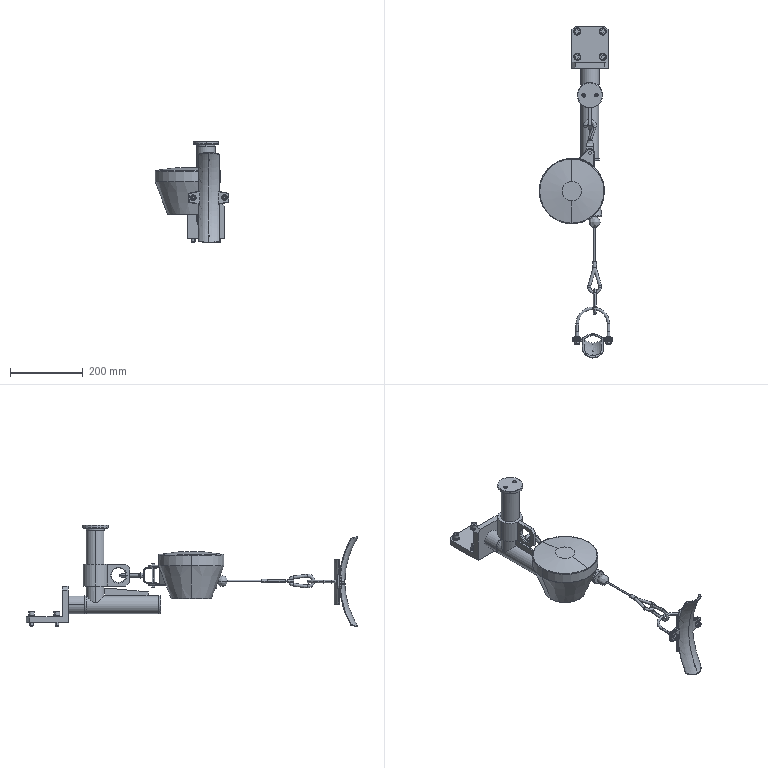Part | SolidWorks | 37 solids | 720 faces | box 203.047 x 914.102 x 280.36 mm | volume 3806317 mm3 | plane 252 | cylinder 248 | cone 84 | spline 74 | torus 40 | sphere 22 | commonest cylinder face diameters 2 x34 8 x25 10 x22 4 x16 11 x16 50 x13